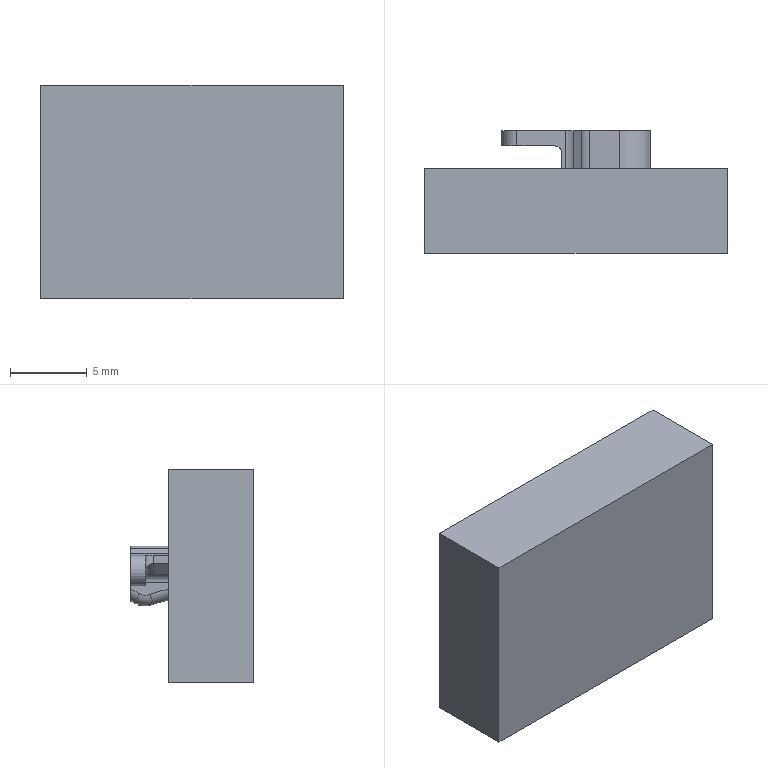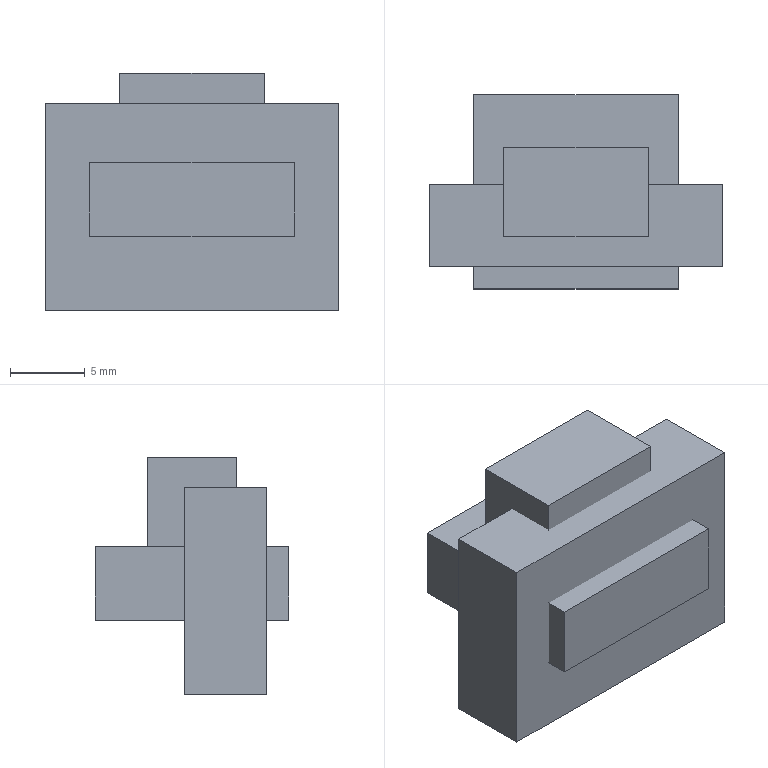CAM job | NX | 3+2 milling, drilling | part box 19.7 x 8 x 13.91 mm | stock box 19.7 x 13 x 15.91 mm
Tools:
number,name,description,diameter,corner_radius,flute_length,length,flutes
10,D10JING,Milling Tool-5 Parameters,10.0,0.0,50.0,75.0,2
4,D4,Milling Tool-5 Parameters,4.0,0.0,50.0,75.0,2
1,ZXZ,Milling Tool-5 Parameters,6.0,0.0,50.0,75.0,2
11,1.0ZT,Drilling Tool,1.0,0.0,35.0,50.0,2
2,D2,Milling Tool-5 Parameters,2.0,0.0,50.0,75.0,2
5,D1,Milling Tool-5 Parameters,1.0,0.0,50.0,75.0,2
7,D6A45,Milling Tool-5 Parameters,6.0,0.0,50.0,75.0,2
9,D2R0.5,Milling Tool-5 Parameters,2.0,0.5,50.0,75.0,2
3,D3,Milling Tool-5 Parameters,3.0,0.0,50.0,75.0,2
Operations:
program,operation,operation_type,tool,method,geometry_group,spindle_rpm,surface_speed,feed_per_tooth,feed_cut,feed_plunge,cut_length_mm,path_length_mm,cut_time_min,machine_time_min
1,FLOOR_WALL,VolumeBased25DMillingOperation,D10JING,METHOD,A,5000.0,157.0,0.125,1250.0,100.0,90.007,144.007,0.072,0.0774
1,DRILLING,Operation,ZXZ,METHOD,A,5000.0,94.0,0.025,250.0,0.0,3.6,67.2,0.0144,0.0208
1,DRILLING_COPY,Operation,1.0ZT,METHOD,A,2000.0,6.0,0.025,100.0,0.0,10.3,80.601,0.103,0.11
1,CAVITY_MILL_1,CavityMilling,D4,METHOD,A,5500.0,69.0,0.1636,1800.0,100.0,8646.731,8981.223,4.804,4.837
1,ZLEVEL_PROFILE,ZLevelMilling,D4,METHOD,A,5000.0,62.0,0.2,2000.0,1000.0,2814.468,2879.468,1.413,1.419
1,ZLEVEL_PROFILE_COPY,ZLevelMilling,D4,METHOD,A,7000.0,87.0,0.0857,1200.0,1000.0,42.402,111.402,0.0358,0.0427
1,ZLEVEL_PROFILE_COPY_1,ZLevelMilling,D2,METHOD,A,6500.0,40.0,0.0923,1200.0,1000.0,846.515,1502.496,0.7325,0.7981
1,ZLEVEL_PROFILE_COPY_1_COPY,ZLevelMilling,D1,METHOD,A,7000.0,21.0,0.0607,850.0,1000.0,675.294,1093.375,0.7803,0.8222
1,PLANAR_MILL,PlanarMilling,D6A45,METHOD,A,7500.0,141.0,0.0833,1250.0,100.0,35.649,93.649,0.0285,0.0343
2夹具,FLOOR_WALL_1,VolumeBased25DMillingOperation,D1,METHOD,B,9500.0,29.0,0.0658,1250.0,100.0,1236.624,1314.43,0.9893,0.9971
2夹具,PLANAR_MILL_COPY,PlanarMilling,D6A45,METHOD,B,7500.0,141.0,0.0833,1250.0,100.0,33.229,90.229,0.0266,0.0323
2夹具,刀补,VolumeBased25DMillingOperation,D1,METHOD,B,9500.0,29.0,0.0526,1000.0,100.0,23.526,89.526,0.0235,0.0301
3,FLOOR_WALL_COPY,VolumeBased25DMillingOperation,D10JING,METHOD,C,5000.0,157.0,0.125,1250.0,100.0,1014.4,3322.109,0.8115,1.042
3,PLANAR_MILL_COPY_1,PlanarMilling,D6A45,METHOD,C,7500.0,141.0,0.0833,1250.0,100.0,35.649,93.649,0.0285,0.0343
4,CAVITY_MILL,CavityMilling,D3,METHOD,D,5000.0,47.0,0.15,1500.0,1000.0,2240.317,9677.275,1.621,2.365
4,CAVITY_MILL_COPY,CavityMilling,D1,METHOD,D,6000.0,18.0,0.0708,850.0,1000.0,1495.91,1794.342,1.701,1.731
4,FIXED_CONTOUR,SurfaceContour,D2R0.5,METHOD,D,6500.0,61.0,0.1154,1500.0,1000.0,740.733,795.133,0.4953,0.5008
4,FIXED_CONTOUR_COPY,SurfaceContour,D2R0.5,METHOD,D,6500.0,61.0,0.1154,1500.0,1000.0,341.543,410.257,0.2374,0.2443
4,FIXED_CONTOUR_COPY_COPY,SurfaceContour,D2R0.5,METHOD,D,6500.0,61.0,0.1154,1500.0,1000.0,78.471,135.671,0.0538,0.0595